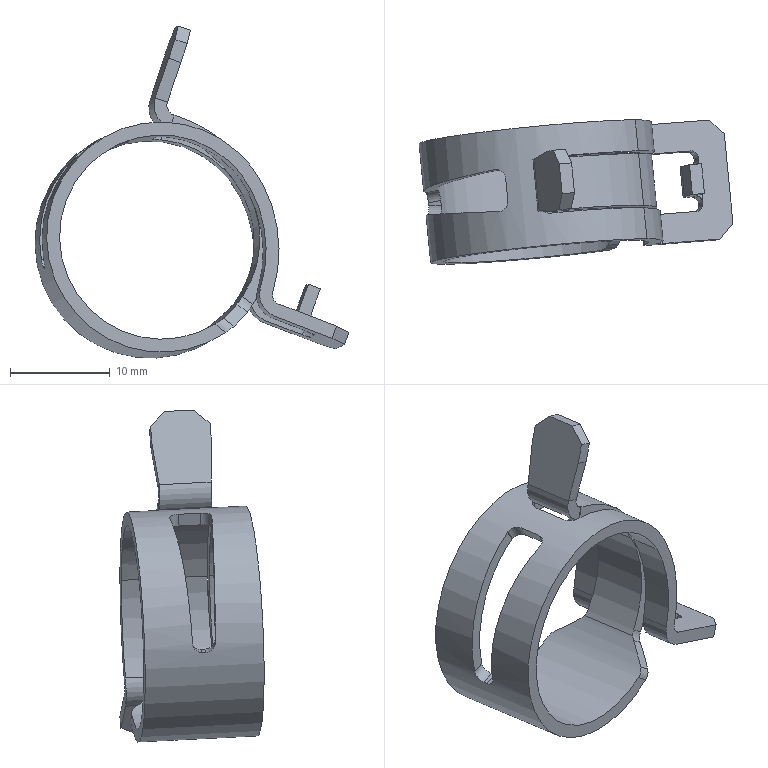Part | SolidWorks | features BaseBody 1 | 1 solid | 74 faces | box 31.483 x 14.462 x 33.309 mm | volume 1146 mm3 | plane 40 | cylinder 31 | spline 3 | commonest cylinder face diameters 2 x12 3 x4 4.6 x4 26 x3 28.6 x3 20.5 x2